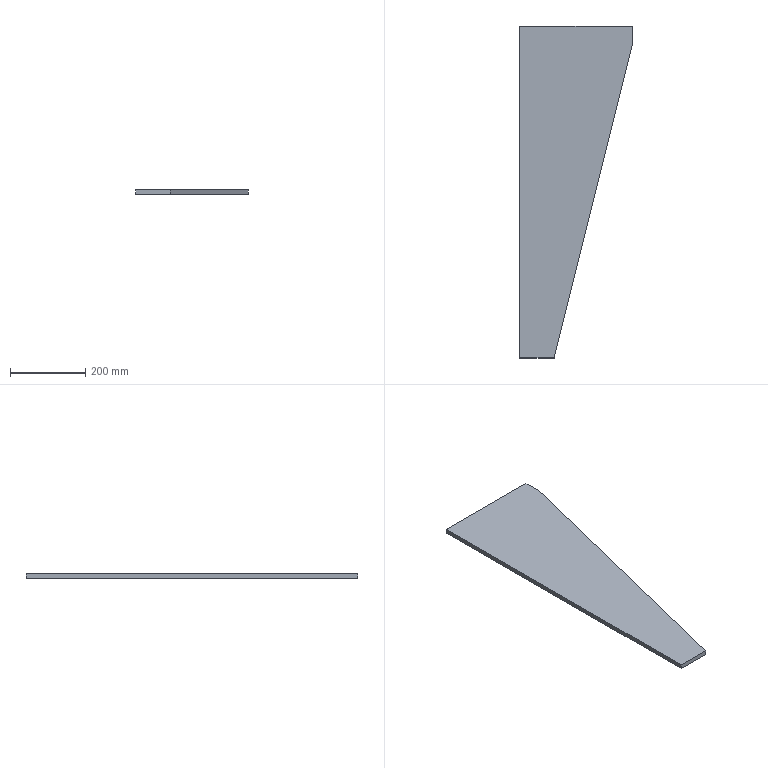Part | SolidWorks | features Extrusion 1 | 1 solid | 7 faces | box 300 x 885 x 12 mm | volume 2143920 mm3 | plane 7
STEP:
#1=CARTESIAN_POINT('',(0.,0.,0.));
#2=VERTEX_POINT('',#1);
#3=CARTESIAN_POINT('',(92.,0.,0.));
#4=VERTEX_POINT('',#3);
#5=CARTESIAN_POINT('',(92.,0.,0.));
#6=DIRECTION('',(1.,0.,0.));
#7=VECTOR('',#6,1000.);
#8=LINE('',#5,#7);
#9=EDGE_CURVE('',#2,#4,#8,.T.);
#10=ORIENTED_EDGE('',*,*,#9,.T.);
#11=CARTESIAN_POINT('',(92.,0.,12.));
#12=VERTEX_POINT('',#11);
#13=CARTESIAN_POINT('',(92.,0.,12.));
#14=DIRECTION('',(0.,0.,-1.));
#15=VECTOR('',#14,1000.);
#16=LINE('',#13,#15);
#17=EDGE_CURVE('',#12,#4,#16,.T.);
#18=ORIENTED_EDGE('',*,*,#17,.F.);
#19=CARTESIAN_POINT('',(0.,0.,12.));
#20=VERTEX_POINT('',#19);
#21=CARTESIAN_POINT('',(92.,0.,12.));
#22=DIRECTION('',(1.,0.,0.));
#23=VECTOR('',#22,1000.);
#24=LINE('',#21,#23);
#25=EDGE_CURVE('',#20,#12,#24,.T.);
#26=ORIENTED_EDGE('',*,*,#25,.F.);
#27=CARTESIAN_POINT('',(0.,0.,12.));
#28=DIRECTION('',(0.,0.,-1.));
#29=VECTOR('',#28,1000.);
#30=LINE('',#27,#29);
#31=EDGE_CURVE('',#20,#2,#30,.T.);
#32=ORIENTED_EDGE('',*,*,#31,.T.);
#33=EDGE_LOOP('',(#10,#18,#26,#32));
#34=FACE_OUTER_BOUND('',#33,.T.);
#35=CARTESIAN_POINT('',(92.,0.,12.));
#36=DIRECTION('',(0.,1.,0.));
#37=DIRECTION('',(-1.,0.,0.));
#38=AXIS2_PLACEMENT_3D('',#35,#36,#37);
#39=PLANE('',#38);
#40=ADVANCED_FACE('',(#34),#39,.F.);
#41=CARTESIAN_POINT('',(300.,835.,0.));
#42=VERTEX_POINT('',#41);
#43=CARTESIAN_POINT('',(300.,835.,0.));
#44=DIRECTION('',(0.2417,0.9703,0.));
#45=VECTOR('',#44,1000.);
#46=LINE('',#43,#45);
#47=EDGE_CURVE('',#4,#42,#46,.T.);
#48=ORIENTED_EDGE('',*,*,#47,.T.);
#49=CARTESIAN_POINT('',(300.,835.,12.));
#50=VERTEX_POINT('',#49);
#51=CARTESIAN_POINT('',(300.,835.,12.));
#52=DIRECTION('',(0.,0.,-1.));
#53=VECTOR('',#52,1000.);
#54=LINE('',#51,#53);
#55=EDGE_CURVE('',#50,#42,#54,.T.);
#56=ORIENTED_EDGE('',*,*,#55,.F.);
#57=CARTESIAN_POINT('',(300.,835.,12.));
#58=DIRECTION('',(0.2417,0.9703,0.));
#59=VECTOR('',#58,1000.);
#60=LINE('',#57,#59);
#61=EDGE_CURVE('',#12,#50,#60,.T.);
#62=ORIENTED_EDGE('',*,*,#61,.F.);
#63=ORIENTED_EDGE('',*,*,#17,.T.);
#64=EDGE_LOOP('',(#48,#56,#62,#63));
#65=FACE_OUTER_BOUND('',#64,.T.);
#66=CARTESIAN_POINT('',(300.,835.,12.));
#67=DIRECTION('',(-0.9703,0.2417,0.));
#68=DIRECTION('',(-0.2417,-0.9703,0.));
#69=AXIS2_PLACEMENT_3D('',#66,#67,#68);
#70=PLANE('',#69);
#71=ADVANCED_FACE('',(#65),#70,.F.);
#72=CARTESIAN_POINT('',(300.,885.,0.));
#73=VERTEX_POINT('',#72);
#74=CARTESIAN_POINT('',(300.,885.,0.));
#75=DIRECTION('',(0.,1.,0.));
#76=VECTOR('',#75,1000.);
#77=LINE('',#74,#76);
#78=EDGE_CURVE('',#42,#73,#77,.T.);
#79=ORIENTED_EDGE('',*,*,#78,.T.);
#80=CARTESIAN_POINT('',(300.,885.,12.));
#81=VERTEX_POINT('',#80);
#82=CARTESIAN_POINT('',(300.,885.,12.));
#83=DIRECTION('',(0.,0.,-1.));
#84=VECTOR('',#83,1000.);
#85=LINE('',#82,#84);
#86=EDGE_CURVE('',#81,#73,#85,.T.);
#87=ORIENTED_EDGE('',*,*,#86,.F.);
#88=CARTESIAN_POINT('',(300.,885.,12.));
#89=DIRECTION('',(0.,1.,0.));
#90=VECTOR('',#89,1000.);
#91=LINE('',#88,#90);
#92=EDGE_CURVE('',#50,#81,#91,.T.);
#93=ORIENTED_EDGE('',*,*,#92,.F.);
#94=ORIENTED_EDGE('',*,*,#55,.T.);
#95=EDGE_LOOP('',(#79,#87,#93,#94));
#96=FACE_OUTER_BOUND('',#95,.T.);
#97=CARTESIAN_POINT('',(300.,885.,12.));
#98=DIRECTION('',(-1.,0.,0.));
#99=DIRECTION('',(0.,0.,1.));
#100=AXIS2_PLACEMENT_3D('',#97,#98,#99);
#101=PLANE('',#100);
#102=ADVANCED_FACE('',(#96),#101,.F.);
#103=CARTESIAN_POINT('',(0.,885.,0.));
#104=VERTEX_POINT('',#103);
#105=CARTESIAN_POINT('',(0.,885.,0.));
#106=DIRECTION('',(-1.,0.,0.));
#107=VECTOR('',#106,1000.);
#108=LINE('',#105,#107);
#109=EDGE_CURVE('',#73,#104,#108,.T.);
#110=ORIENTED_EDGE('',*,*,#109,.T.);
#111=CARTESIAN_POINT('',(0.,885.,12.));
#112=VERTEX_POINT('',#111);
#113=CARTESIAN_POINT('',(0.,885.,12.));
#114=DIRECTION('',(0.,0.,-1.));
#115=VECTOR('',#114,1000.);
#116=LINE('',#113,#115);
#117=EDGE_CURVE('',#112,#104,#116,.T.);
#118=ORIENTED_EDGE('',*,*,#117,.F.);
#119=CARTESIAN_POINT('',(0.,885.,12.));
#120=DIRECTION('',(-1.,0.,0.));
#121=VECTOR('',#120,1000.);
#122=LINE('',#119,#121);
#123=EDGE_CURVE('',#81,#112,#122,.T.);
#124=ORIENTED_EDGE('',*,*,#123,.F.);
#125=ORIENTED_EDGE('',*,*,#86,.T.);
#126=EDGE_LOOP('',(#110,#118,#124,#125));
#127=FACE_OUTER_BOUND('',#126,.T.);
#128=CARTESIAN_POINT('',(0.,885.,12.));
#129=DIRECTION('',(0.,-1.,0.));
#130=DIRECTION('',(0.,0.,-1.));
#131=AXIS2_PLACEMENT_3D('',#128,#129,#130);
#132=PLANE('',#131);
#133=ADVANCED_FACE('',(#127),#132,.F.);
#134=CARTESIAN_POINT('',(0.,0.,0.));
#135=DIRECTION('',(0.,-1.,0.));
#136=VECTOR('',#135,1000.);
#137=LINE('',#134,#136);
#138=EDGE_CURVE('',#104,#2,#137,.T.);
#139=ORIENTED_EDGE('',*,*,#138,.T.);
#140=ORIENTED_EDGE('',*,*,#31,.F.);
#141=CARTESIAN_POINT('',(0.,0.,12.));
#142=DIRECTION('',(0.,-1.,0.));
#143=VECTOR('',#142,1000.);
#144=LINE('',#141,#143);
#145=EDGE_CURVE('',#112,#20,#144,.T.);
#146=ORIENTED_EDGE('',*,*,#145,.F.);
#147=ORIENTED_EDGE('',*,*,#117,.T.);
#148=EDGE_LOOP('',(#139,#140,#146,#147));
#149=FACE_OUTER_BOUND('',#148,.T.);
#150=CARTESIAN_POINT('',(0.,0.,12.));
#151=DIRECTION('',(1.,0.,0.));
#152=DIRECTION('',(0.,0.,-1.));
#153=AXIS2_PLACEMENT_3D('',#150,#151,#152);
#154=PLANE('',#153);
#155=ADVANCED_FACE('',(#149),#154,.F.);
#156=ORIENTED_EDGE('',*,*,#25,.T.);
#157=ORIENTED_EDGE('',*,*,#61,.T.);
#158=ORIENTED_EDGE('',*,*,#92,.T.);
#159=ORIENTED_EDGE('',*,*,#123,.T.);
#160=ORIENTED_EDGE('',*,*,#145,.T.);
#161=EDGE_LOOP('',(#156,#157,#158,#159,#160));
#162=FACE_OUTER_BOUND('',#161,.T.);
#163=CARTESIAN_POINT('',(0.,0.,12.));
#164=DIRECTION('',(0.,0.,-1.));
#165=DIRECTION('',(-1.,0.,0.));
#166=AXIS2_PLACEMENT_3D('',#163,#164,#165);
#167=PLANE('',#166);
#168=ADVANCED_FACE('',(#162),#167,.F.);
#169=ORIENTED_EDGE('',*,*,#9,.F.);
#170=ORIENTED_EDGE('',*,*,#138,.F.);
#171=ORIENTED_EDGE('',*,*,#109,.F.);
#172=ORIENTED_EDGE('',*,*,#78,.F.);
#173=ORIENTED_EDGE('',*,*,#47,.F.);
#174=EDGE_LOOP('',(#169,#170,#171,#172,#173));
#175=FACE_OUTER_BOUND('',#174,.T.);
#176=CARTESIAN_POINT('',(0.,0.,0.));
#177=DIRECTION('',(0.,0.,-1.));
#178=DIRECTION('',(-1.,0.,0.));
#179=AXIS2_PLACEMENT_3D('',#176,#177,#178);
#180=PLANE('',#179);
#181=ADVANCED_FACE('',(#175),#180,.T.);
#182=CLOSED_SHELL('',(#40,#71,#102,#133,#155,#168,#181));
#183=MANIFOLD_SOLID_BREP('',#182);
#184=CARTESIAN_POINT('',(0.,0.,0.));
#185=DIRECTION('',(0.,0.,1.));
#186=DIRECTION('',(1.,0.,0.));
#187=AXIS2_PLACEMENT_3D('',#184,#185,#186);
#188=(LENGTH_UNIT()NAMED_UNIT(*)SI_UNIT(.MILLI.,.METRE.));
#189=UNCERTAINTY_MEASURE_WITH_UNIT(LENGTH_MEASURE(0.00001),#188,'','');
#190=(NAMED_UNIT(*)PLANE_ANGLE_UNIT()SI_UNIT($,.RADIAN.));
#191=(NAMED_UNIT(*)SI_UNIT($,.STERADIAN.)SOLID_ANGLE_UNIT());
#192=(GEOMETRIC_REPRESENTATION_CONTEXT(3)GLOBAL_UNCERTAINTY_ASSIGNED_CONTEXT((#189))GLOBAL_UNIT_ASSIGNED_CONTEXT((#188,#190,#191))REPRESENTATION_CONTEXT('',''));
#193=ADVANCED_BREP_SHAPE_REPRESENTATION('',(#183,#187),#192);